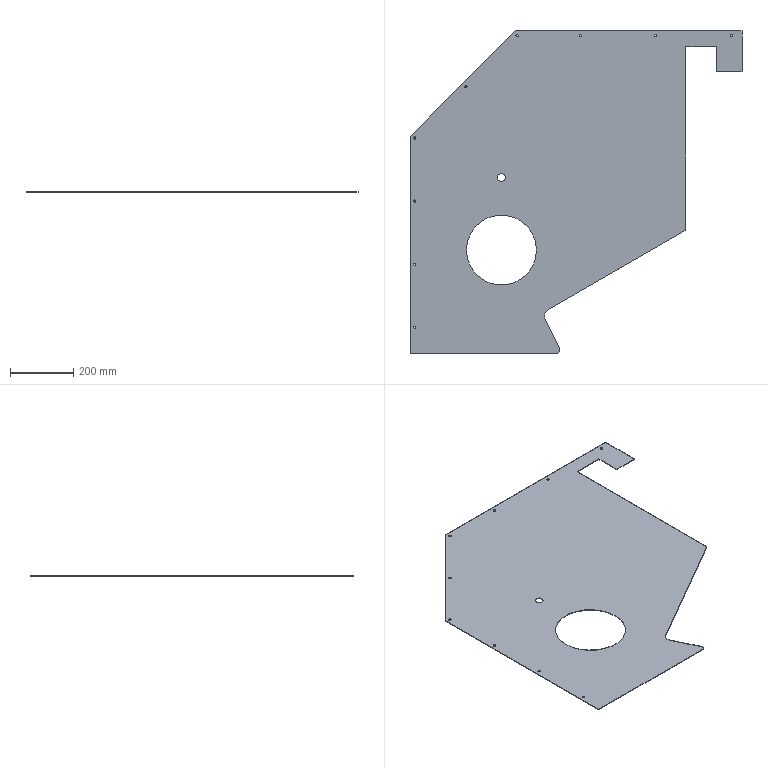Part | STEP file | Center Shaft Plate 2 | 1 solid | 38 faces | box 1053 x 1022 x 2 mm | volume 1400799 mm3 | cylinder 25 | plane 13 | commonest cylinder face diameters 7 x18 20 x2 25 x2 222 x2 40 x1
STEP:
#1=CARTESIAN_POINT('',(-529.64,-129.457,-2.));
#2=VERTEX_POINT('',#1);
#3=CARTESIAN_POINT('',(-519.64,-119.457,-2.));
#4=VERTEX_POINT('',#3);
#5=CARTESIAN_POINT('',(-529.64,-119.457,-2.));
#6=DIRECTION('',(0.,0.,1.));
#7=DIRECTION('',(1.,0.,0.));
#8=AXIS2_PLACEMENT_3D('',#5,#6,#7);
#9=CIRCLE('',#8,10.);
#10=EDGE_CURVE('',#2,#4,#9,.T.);
#11=ORIENTED_EDGE('',*,*,#10,.T.);
#12=CARTESIAN_POINT('',(-519.64,-119.457,0.));
#13=VERTEX_POINT('',#12);
#14=CARTESIAN_POINT('',(-519.64,-119.457,-2.));
#15=DIRECTION('',(0.,0.,1.));
#16=VECTOR('',#15,1000.);
#17=LINE('',#14,#16);
#18=EDGE_CURVE('',#4,#13,#17,.T.);
#19=ORIENTED_EDGE('',*,*,#18,.T.);
#20=CARTESIAN_POINT('',(-529.64,-129.457,0.));
#21=VERTEX_POINT('',#20);
#22=CARTESIAN_POINT('',(-529.64,-119.457,0.));
#23=DIRECTION('',(0.,0.,1.));
#24=DIRECTION('',(1.,0.,0.));
#25=AXIS2_PLACEMENT_3D('',#22,#23,#24);
#26=CIRCLE('',#25,10.);
#27=EDGE_CURVE('',#21,#13,#26,.T.);
#28=ORIENTED_EDGE('',*,*,#27,.F.);
#29=CARTESIAN_POINT('',(-529.64,-129.457,-2.));
#30=DIRECTION('',(0.,0.,-1.));
#31=VECTOR('',#30,1000.);
#32=LINE('',#29,#31);
#33=EDGE_CURVE('',#21,#2,#32,.T.);
#34=ORIENTED_EDGE('',*,*,#33,.T.);
#35=EDGE_LOOP('',(#11,#19,#28,#34));
#36=FACE_OUTER_BOUND('',#35,.T.);
#37=CARTESIAN_POINT('',(-529.64,-119.457,-2.));
#38=DIRECTION('',(0.,0.,1.));
#39=DIRECTION('',(1.,0.,0.));
#40=AXIS2_PLACEMENT_3D('',#37,#38,#39);
#41=CYLINDRICAL_SURFACE('',#40,10.);
#42=ADVANCED_FACE('',(#36),#41,.T.);
#43=CARTESIAN_POINT('',(-815.802,197.43,-2.));
#44=VERTEX_POINT('',#43);
#45=CARTESIAN_POINT('',(-593.802,197.43,-2.));
#46=VERTEX_POINT('',#45);
#47=CARTESIAN_POINT('',(-704.802,197.43,-2.));
#48=DIRECTION('',(0.,0.,1.));
#49=DIRECTION('',(1.,0.,0.));
#50=AXIS2_PLACEMENT_3D('',#47,#48,#49);
#51=CIRCLE('',#50,111.);
#52=EDGE_CURVE('',#44,#46,#51,.T.);
#53=ORIENTED_EDGE('',*,*,#52,.F.);
#54=CARTESIAN_POINT('',(-815.802,197.43,0.));
#55=VERTEX_POINT('',#54);
#56=CARTESIAN_POINT('',(-815.802,197.43,-2.));
#57=DIRECTION('',(0.,0.,1.));
#58=VECTOR('',#57,1000.);
#59=LINE('',#56,#58);
#60=EDGE_CURVE('',#44,#55,#59,.T.);
#61=ORIENTED_EDGE('',*,*,#60,.T.);
#62=CARTESIAN_POINT('',(-593.802,197.43,0.));
#63=VERTEX_POINT('',#62);
#64=CARTESIAN_POINT('',(-704.802,197.43,0.));
#65=DIRECTION('',(0.,0.,-1.));
#66=DIRECTION('',(1.,0.,0.));
#67=AXIS2_PLACEMENT_3D('',#64,#65,#66);
#68=CIRCLE('',#67,111.);
#69=EDGE_CURVE('',#63,#55,#68,.T.);
#70=ORIENTED_EDGE('',*,*,#69,.F.);
#71=CARTESIAN_POINT('',(-593.802,197.43,-2.));
#72=DIRECTION('',(0.,0.,1.));
#73=VECTOR('',#72,1000.);
#74=LINE('',#71,#73);
#75=EDGE_CURVE('',#46,#63,#74,.T.);
#76=ORIENTED_EDGE('',*,*,#75,.F.);
#77=EDGE_LOOP('',(#53,#61,#70,#76));
#78=FACE_OUTER_BOUND('',#77,.T.);
#79=CARTESIAN_POINT('',(-704.802,197.43,-2.));
#80=DIRECTION('',(0.,0.,1.));
#81=DIRECTION('',(1.,0.,0.));
#82=AXIS2_PLACEMENT_3D('',#79,#80,#81);
#83=CYLINDRICAL_SURFACE('',#82,111.);
#84=ADVANCED_FACE('',(#78),#83,.F.);
#85=CARTESIAN_POINT('',(-717.302,427.43,-2.));
#86=VERTEX_POINT('',#85);
#87=CARTESIAN_POINT('',(-692.302,427.43,-2.));
#88=VERTEX_POINT('',#87);
#89=CARTESIAN_POINT('',(-704.802,427.43,-2.));
#90=DIRECTION('',(0.,0.,1.));
#91=DIRECTION('',(1.,0.,0.));
#92=AXIS2_PLACEMENT_3D('',#89,#90,#91);
#93=CIRCLE('',#92,12.5);
#94=EDGE_CURVE('',#86,#88,#93,.T.);
#95=ORIENTED_EDGE('',*,*,#94,.F.);
#96=CARTESIAN_POINT('',(-717.302,427.43,0.));
#97=VERTEX_POINT('',#96);
#98=CARTESIAN_POINT('',(-717.302,427.43,-2.));
#99=DIRECTION('',(0.,0.,1.));
#100=VECTOR('',#99,1000.);
#101=LINE('',#98,#100);
#102=EDGE_CURVE('',#86,#97,#101,.T.);
#103=ORIENTED_EDGE('',*,*,#102,.T.);
#104=CARTESIAN_POINT('',(-692.302,427.43,0.));
#105=VERTEX_POINT('',#104);
#106=CARTESIAN_POINT('',(-704.802,427.43,0.));
#107=DIRECTION('',(0.,0.,-1.));
#108=DIRECTION('',(1.,0.,0.));
#109=AXIS2_PLACEMENT_3D('',#106,#107,#108);
#110=CIRCLE('',#109,12.5);
#111=EDGE_CURVE('',#105,#97,#110,.T.);
#112=ORIENTED_EDGE('',*,*,#111,.F.);
#113=CARTESIAN_POINT('',(-692.302,427.43,-2.));
#114=DIRECTION('',(0.,0.,1.));
#115=VECTOR('',#114,1000.);
#116=LINE('',#113,#115);
#117=EDGE_CURVE('',#88,#105,#116,.T.);
#118=ORIENTED_EDGE('',*,*,#117,.F.);
#119=EDGE_LOOP('',(#95,#103,#112,#118));
#120=FACE_OUTER_BOUND('',#119,.T.);
#121=CARTESIAN_POINT('',(-704.802,427.43,-2.));
#122=DIRECTION('',(0.,0.,1.));
#123=DIRECTION('',(1.,0.,0.));
#124=AXIS2_PLACEMENT_3D('',#121,#122,#123);
#125=CYLINDRICAL_SURFACE('',#124,12.5);
#126=ADVANCED_FACE('',(#120),#125,.F.);
#127=CARTESIAN_POINT('',(-983.302,552.785,-2.));
#128=VERTEX_POINT('',#127);
#129=CARTESIAN_POINT('',(-976.302,552.785,-2.));
#130=VERTEX_POINT('',#129);
#131=CARTESIAN_POINT('',(-979.802,552.785,-2.));
#132=DIRECTION('',(0.,0.,1.));
#133=DIRECTION('',(1.,0.,0.));
#134=AXIS2_PLACEMENT_3D('',#131,#132,#133);
#135=CIRCLE('',#134,3.5);
#136=EDGE_CURVE('',#128,#130,#135,.T.);
#137=ORIENTED_EDGE('',*,*,#136,.F.);
#138=CARTESIAN_POINT('',(-983.302,552.785,0.));
#139=VERTEX_POINT('',#138);
#140=CARTESIAN_POINT('',(-983.302,552.785,-10.));
#141=DIRECTION('',(0.,0.,1.));
#142=VECTOR('',#141,1000.);
#143=LINE('',#140,#142);
#144=EDGE_CURVE('',#128,#139,#143,.T.);
#145=ORIENTED_EDGE('',*,*,#144,.T.);
#146=CARTESIAN_POINT('',(-976.302,552.785,0.));
#147=VERTEX_POINT('',#146);
#148=CARTESIAN_POINT('',(-979.802,552.785,0.));
#149=DIRECTION('',(0.,0.,-1.));
#150=DIRECTION('',(1.,0.,0.));
#151=AXIS2_PLACEMENT_3D('',#148,#149,#150);
#152=CIRCLE('',#151,3.5);
#153=EDGE_CURVE('',#147,#139,#152,.T.);
#154=ORIENTED_EDGE('',*,*,#153,.F.);
#155=CARTESIAN_POINT('',(-976.302,552.785,-10.));
#156=DIRECTION('',(0.,0.,1.));
#157=VECTOR('',#156,1000.);
#158=LINE('',#155,#157);
#159=EDGE_CURVE('',#130,#147,#158,.T.);
#160=ORIENTED_EDGE('',*,*,#159,.F.);
#161=EDGE_LOOP('',(#137,#145,#154,#160));
#162=FACE_OUTER_BOUND('',#161,.T.);
#163=CARTESIAN_POINT('',(-979.802,552.785,-10.));
#164=DIRECTION('',(0.,0.,1.));
#165=DIRECTION('',(1.,0.,0.));
#166=AXIS2_PLACEMENT_3D('',#163,#164,#165);
#167=CYLINDRICAL_SURFACE('',#166,3.5);
#168=ADVANCED_FACE('',(#162),#167,.F.);
#169=CARTESIAN_POINT('',(-983.302,-47.215,-2.));
#170=VERTEX_POINT('',#169);
#171=CARTESIAN_POINT('',(-976.302,-47.215,-2.));
#172=VERTEX_POINT('',#171);
#173=CARTESIAN_POINT('',(-979.802,-47.215,-2.));
#174=DIRECTION('',(0.,0.,1.));
#175=DIRECTION('',(1.,0.,0.));
#176=AXIS2_PLACEMENT_3D('',#173,#174,#175);
#177=CIRCLE('',#176,3.5);
#178=EDGE_CURVE('',#170,#172,#177,.T.);
#179=ORIENTED_EDGE('',*,*,#178,.F.);
#180=CARTESIAN_POINT('',(-983.302,-47.215,0.));
#181=VERTEX_POINT('',#180);
#182=CARTESIAN_POINT('',(-983.302,-47.215,-10.));
#183=DIRECTION('',(0.,0.,1.));
#184=VECTOR('',#183,1000.);
#185=LINE('',#182,#184);
#186=EDGE_CURVE('',#170,#181,#185,.T.);
#187=ORIENTED_EDGE('',*,*,#186,.T.);
#188=CARTESIAN_POINT('',(-976.302,-47.215,0.));
#189=VERTEX_POINT('',#188);
#190=CARTESIAN_POINT('',(-979.802,-47.215,0.));
#191=DIRECTION('',(0.,0.,-1.));
#192=DIRECTION('',(1.,0.,0.));
#193=AXIS2_PLACEMENT_3D('',#190,#191,#192);
#194=CIRCLE('',#193,3.5);
#195=EDGE_CURVE('',#189,#181,#194,.T.);
#196=ORIENTED_EDGE('',*,*,#195,.F.);
#197=CARTESIAN_POINT('',(-976.302,-47.215,-10.));
#198=DIRECTION('',(0.,0.,1.));
#199=VECTOR('',#198,1000.);
#200=LINE('',#197,#199);
#201=EDGE_CURVE('',#172,#189,#200,.T.);
#202=ORIENTED_EDGE('',*,*,#201,.F.);
#203=EDGE_LOOP('',(#179,#187,#196,#202));
#204=FACE_OUTER_BOUND('',#203,.T.);
#205=CARTESIAN_POINT('',(-979.802,-47.215,-10.));
#206=DIRECTION('',(0.,0.,1.));
#207=DIRECTION('',(1.,0.,0.));
#208=AXIS2_PLACEMENT_3D('',#205,#206,#207);
#209=CYLINDRICAL_SURFACE('',#208,3.5);
#210=ADVANCED_FACE('',(#204),#209,.F.);
#211=CARTESIAN_POINT('',(-983.302,152.785,-2.));
#212=VERTEX_POINT('',#211);
#213=CARTESIAN_POINT('',(-976.302,152.785,-2.));
#214=VERTEX_POINT('',#213);
#215=CARTESIAN_POINT('',(-979.802,152.785,-2.));
#216=DIRECTION('',(0.,0.,1.));
#217=DIRECTION('',(1.,0.,0.));
#218=AXIS2_PLACEMENT_3D('',#215,#216,#217);
#219=CIRCLE('',#218,3.5);
#220=EDGE_CURVE('',#212,#214,#219,.T.);
#221=ORIENTED_EDGE('',*,*,#220,.F.);
#222=CARTESIAN_POINT('',(-983.302,152.785,0.));
#223=VERTEX_POINT('',#222);
#224=CARTESIAN_POINT('',(-983.302,152.785,-10.));
#225=DIRECTION('',(0.,0.,1.));
#226=VECTOR('',#225,1000.);
#227=LINE('',#224,#226);
#228=EDGE_CURVE('',#212,#223,#227,.T.);
#229=ORIENTED_EDGE('',*,*,#228,.T.);
#230=CARTESIAN_POINT('',(-976.302,152.785,0.));
#231=VERTEX_POINT('',#230);
#232=CARTESIAN_POINT('',(-979.802,152.785,0.));
#233=DIRECTION('',(0.,0.,-1.));
#234=DIRECTION('',(1.,0.,0.));
#235=AXIS2_PLACEMENT_3D('',#232,#233,#234);
#236=CIRCLE('',#235,3.5);
#237=EDGE_CURVE('',#231,#223,#236,.T.);
#238=ORIENTED_EDGE('',*,*,#237,.F.);
#239=CARTESIAN_POINT('',(-976.302,152.785,-10.));
#240=DIRECTION('',(0.,0.,1.));
#241=VECTOR('',#240,1000.);
#242=LINE('',#239,#241);
#243=EDGE_CURVE('',#214,#231,#242,.T.);
#244=ORIENTED_EDGE('',*,*,#243,.F.);
#245=EDGE_LOOP('',(#221,#229,#238,#244));
#246=FACE_OUTER_BOUND('',#245,.T.);
#247=CARTESIAN_POINT('',(-979.802,152.785,-10.));
#248=DIRECTION('',(0.,0.,1.));
#249=DIRECTION('',(1.,0.,0.));
#250=AXIS2_PLACEMENT_3D('',#247,#248,#249);
#251=CYLINDRICAL_SURFACE('',#250,3.5);
#252=ADVANCED_FACE('',(#246),#251,.F.);
#253=CARTESIAN_POINT('',(-983.302,352.785,-2.));
#254=VERTEX_POINT('',#253);
#255=CARTESIAN_POINT('',(-976.302,352.785,-2.));
#256=VERTEX_POINT('',#255);
#257=CARTESIAN_POINT('',(-979.802,352.785,-2.));
#258=DIRECTION('',(0.,0.,1.));
#259=DIRECTION('',(1.,0.,0.));
#260=AXIS2_PLACEMENT_3D('',#257,#258,#259);
#261=CIRCLE('',#260,3.5);
#262=EDGE_CURVE('',#254,#256,#261,.T.);
#263=ORIENTED_EDGE('',*,*,#262,.F.);
#264=CARTESIAN_POINT('',(-983.302,352.785,0.));
#265=VERTEX_POINT('',#264);
#266=CARTESIAN_POINT('',(-983.302,352.785,-10.));
#267=DIRECTION('',(0.,0.,1.));
#268=VECTOR('',#267,1000.);
#269=LINE('',#266,#268);
#270=EDGE_CURVE('',#254,#265,#269,.T.);
#271=ORIENTED_EDGE('',*,*,#270,.T.);
#272=CARTESIAN_POINT('',(-976.302,352.785,0.));
#273=VERTEX_POINT('',#272);
#274=CARTESIAN_POINT('',(-979.802,352.785,0.));
#275=DIRECTION('',(0.,0.,-1.));
#276=DIRECTION('',(1.,0.,0.));
#277=AXIS2_PLACEMENT_3D('',#274,#275,#276);
#278=CIRCLE('',#277,3.5);
#279=EDGE_CURVE('',#273,#265,#278,.T.);
#280=ORIENTED_EDGE('',*,*,#279,.F.);
#281=CARTESIAN_POINT('',(-976.302,352.785,-10.));
#282=DIRECTION('',(0.,0.,1.));
#283=VECTOR('',#282,1000.);
#284=LINE('',#281,#283);
#285=EDGE_CURVE('',#256,#273,#284,.T.);
#286=ORIENTED_EDGE('',*,*,#285,.F.);
#287=EDGE_LOOP('',(#263,#271,#280,#286));
#288=FACE_OUTER_BOUND('',#287,.T.);
#289=CARTESIAN_POINT('',(-979.802,352.785,-10.));
#290=DIRECTION('',(0.,0.,1.));
#291=DIRECTION('',(1.,0.,0.));
#292=AXIS2_PLACEMENT_3D('',#289,#290,#291);
#293=CYLINDRICAL_SURFACE('',#292,3.5);
#294=ADVANCED_FACE('',(#288),#293,.F.);
#295=CARTESIAN_POINT('',(-658.658,877.43,-2.));
#296=VERTEX_POINT('',#295);
#297=CARTESIAN_POINT('',(-651.658,877.43,-2.));
#298=VERTEX_POINT('',#297);
#299=CARTESIAN_POINT('',(-655.158,877.43,-2.));
#300=DIRECTION('',(0.,0.,1.));
#301=DIRECTION('',(1.,0.,0.));
#302=AXIS2_PLACEMENT_3D('',#299,#300,#301);
#303=CIRCLE('',#302,3.5);
#304=EDGE_CURVE('',#296,#298,#303,.T.);
#305=ORIENTED_EDGE('',*,*,#304,.F.);
#306=CARTESIAN_POINT('',(-658.658,877.43,0.));
#307=VERTEX_POINT('',#306);
#308=CARTESIAN_POINT('',(-658.658,877.43,-10.));
#309=DIRECTION('',(0.,0.,1.));
#310=VECTOR('',#309,1000.);
#311=LINE('',#308,#310);
#312=EDGE_CURVE('',#296,#307,#311,.T.);
#313=ORIENTED_EDGE('',*,*,#312,.T.);
#314=CARTESIAN_POINT('',(-651.658,877.43,0.));
#315=VERTEX_POINT('',#314);
#316=CARTESIAN_POINT('',(-655.158,877.43,0.));
#317=DIRECTION('',(0.,0.,-1.));
#318=DIRECTION('',(1.,0.,0.));
#319=AXIS2_PLACEMENT_3D('',#316,#317,#318);
#320=CIRCLE('',#319,3.5);
#321=EDGE_CURVE('',#315,#307,#320,.T.);
#322=ORIENTED_EDGE('',*,*,#321,.F.);
#323=CARTESIAN_POINT('',(-651.658,877.43,-10.));
#324=DIRECTION('',(0.,0.,1.));
#325=VECTOR('',#324,1000.);
#326=LINE('',#323,#325);
#327=EDGE_CURVE('',#298,#315,#326,.T.);
#328=ORIENTED_EDGE('',*,*,#327,.F.);
#329=EDGE_LOOP('',(#305,#313,#322,#328));
#330=FACE_OUTER_BOUND('',#329,.T.);
#331=CARTESIAN_POINT('',(-655.158,877.43,-10.));
#332=DIRECTION('',(0.,0.,1.));
#333=DIRECTION('',(1.,0.,0.));
#334=AXIS2_PLACEMENT_3D('',#331,#332,#333);
#335=CYLINDRICAL_SURFACE('',#334,3.5);
#336=ADVANCED_FACE('',(#330),#335,.F.);
#337=CARTESIAN_POINT('',(-820.98,715.107,-2.));
#338=VERTEX_POINT('',#337);
#339=CARTESIAN_POINT('',(-813.98,715.107,-2.));
#340=VERTEX_POINT('',#339);
#341=CARTESIAN_POINT('',(-817.48,715.107,-2.));
#342=DIRECTION('',(0.,0.,1.));
#343=DIRECTION('',(1.,0.,0.));
#344=AXIS2_PLACEMENT_3D('',#341,#342,#343);
#345=CIRCLE('',#344,3.5);
#346=EDGE_CURVE('',#338,#340,#345,.T.);
#347=ORIENTED_EDGE('',*,*,#346,.F.);
#348=CARTESIAN_POINT('',(-820.98,715.107,0.));
#349=VERTEX_POINT('',#348);
#350=CARTESIAN_POINT('',(-820.98,715.107,-10.));
#351=DIRECTION('',(0.,0.,1.));
#352=VECTOR('',#351,1000.);
#353=LINE('',#350,#352);
#354=EDGE_CURVE('',#338,#349,#353,.T.);
#355=ORIENTED_EDGE('',*,*,#354,.T.);
#356=CARTESIAN_POINT('',(-813.98,715.107,0.));
#357=VERTEX_POINT('',#356);
#358=CARTESIAN_POINT('',(-817.48,715.107,0.));
#359=DIRECTION('',(0.,0.,-1.));
#360=DIRECTION('',(1.,0.,0.));
#361=AXIS2_PLACEMENT_3D('',#358,#359,#360);
#362=CIRCLE('',#361,3.5);
#363=EDGE_CURVE('',#357,#349,#362,.T.);
#364=ORIENTED_EDGE('',*,*,#363,.F.);
#365=CARTESIAN_POINT('',(-813.98,715.107,-10.));
#366=DIRECTION('',(0.,0.,1.));
#367=VECTOR('',#366,1000.);
#368=LINE('',#365,#367);
#369=EDGE_CURVE('',#340,#357,#368,.T.);
#370=ORIENTED_EDGE('',*,*,#369,.F.);
#371=EDGE_LOOP('',(#347,#355,#364,#370));
#372=FACE_OUTER_BOUND('',#371,.T.);
#373=CARTESIAN_POINT('',(-817.48,715.107,-10.));
#374=DIRECTION('',(0.,0.,1.));
#375=DIRECTION('',(1.,0.,0.));
#376=AXIS2_PLACEMENT_3D('',#373,#374,#375);
#377=CYLINDRICAL_SURFACE('',#376,3.5);
#378=ADVANCED_FACE('',(#372),#377,.F.);
#379=CARTESIAN_POINT('',(-458.658,877.43,-2.));
#380=VERTEX_POINT('',#379);
#381=CARTESIAN_POINT('',(-451.658,877.43,-2.));
#382=VERTEX_POINT('',#381);
#383=CARTESIAN_POINT('',(-455.158,877.43,-2.));
#384=DIRECTION('',(0.,0.,1.));
#385=DIRECTION('',(1.,0.,0.));
#386=AXIS2_PLACEMENT_3D('',#383,#384,#385);
#387=CIRCLE('',#386,3.5);
#388=EDGE_CURVE('',#380,#382,#387,.T.);
#389=ORIENTED_EDGE('',*,*,#388,.F.);
#390=CARTESIAN_POINT('',(-458.658,877.43,0.));
#391=VERTEX_POINT('',#390);
#392=CARTESIAN_POINT('',(-458.658,877.43,-10.));
#393=DIRECTION('',(0.,0.,1.));
#394=VECTOR('',#393,1000.);
#395=LINE('',#392,#394);
#396=EDGE_CURVE('',#380,#391,#395,.T.);
#397=ORIENTED_EDGE('',*,*,#396,.T.);
#398=CARTESIAN_POINT('',(-451.658,877.43,0.));
#399=VERTEX_POINT('',#398);
#400=CARTESIAN_POINT('',(-455.158,877.43,0.));
#401=DIRECTION('',(0.,0.,-1.));
#402=DIRECTION('',(1.,0.,0.));
#403=AXIS2_PLACEMENT_3D('',#400,#401,#402);
#404=CIRCLE('',#403,3.5);
#405=EDGE_CURVE('',#399,#391,#404,.T.);
#406=ORIENTED_EDGE('',*,*,#405,.F.);
#407=CARTESIAN_POINT('',(-451.658,877.43,-10.));
#408=DIRECTION('',(0.,0.,1.));
#409=VECTOR('',#408,1000.);
#410=LINE('',#407,#409);
#411=EDGE_CURVE('',#382,#399,#410,.T.);
#412=ORIENTED_EDGE('',*,*,#411,.F.);
#413=EDGE_LOOP('',(#389,#397,#406,#412));
#414=FACE_OUTER_BOUND('',#413,.T.);
#415=CARTESIAN_POINT('',(-455.158,877.43,-10.));
#416=DIRECTION('',(0.,0.,1.));
#417=DIRECTION('',(1.,0.,0.));
#418=AXIS2_PLACEMENT_3D('',#415,#416,#417);
#419=CYLINDRICAL_SURFACE('',#418,3.5);
#420=ADVANCED_FACE('',(#414),#419,.F.);
#421=CARTESIAN_POINT('',(-218.658,877.43,-2.));
#422=VERTEX_POINT('',#421);
#423=CARTESIAN_POINT('',(-211.658,877.43,-2.));
#424=VERTEX_POINT('',#423);
#425=CARTESIAN_POINT('',(-215.158,877.43,-2.));
#426=DIRECTION('',(0.,0.,1.));
#427=DIRECTION('',(1.,0.,0.));
#428=AXIS2_PLACEMENT_3D('',#425,#426,#427);
#429=CIRCLE('',#428,3.5);
#430=EDGE_CURVE('',#422,#424,#429,.T.);
#431=ORIENTED_EDGE('',*,*,#430,.F.);
#432=CARTESIAN_POINT('',(-218.658,877.43,0.));
#433=VERTEX_POINT('',#432);
#434=CARTESIAN_POINT('',(-218.658,877.43,-10.));
#435=DIRECTION('',(0.,0.,1.));
#436=VECTOR('',#435,1000.);
#437=LINE('',#434,#436);
#438=EDGE_CURVE('',#422,#433,#437,.T.);
#439=ORIENTED_EDGE('',*,*,#438,.T.);
#440=CARTESIAN_POINT('',(-211.658,877.43,0.));
#441=VERTEX_POINT('',#440);
#442=CARTESIAN_POINT('',(-215.158,877.43,0.));
#443=DIRECTION('',(0.,0.,-1.));
#444=DIRECTION('',(1.,0.,0.));
#445=AXIS2_PLACEMENT_3D('',#442,#443,#444);
#446=CIRCLE('',#445,3.5);
#447=EDGE_CURVE('',#441,#433,#446,.T.);
#448=ORIENTED_EDGE('',*,*,#447,.F.);
#449=CARTESIAN_POINT('',(-211.658,877.43,-10.));
#450=DIRECTION('',(0.,0.,1.));
#451=VECTOR('',#450,1000.);
#452=LINE('',#449,#451);
#453=EDGE_CURVE('',#424,#441,#452,.T.);
#454=ORIENTED_EDGE('',*,*,#453,.F.);
#455=EDGE_LOOP('',(#431,#439,#448,#454));
#456=FACE_OUTER_BOUND('',#455,.T.);
#457=CARTESIAN_POINT('',(-215.158,877.43,-10.));
#458=DIRECTION('',(0.,0.,1.));
#459=DIRECTION('',(1.,0.,0.));
#460=AXIS2_PLACEMENT_3D('',#457,#458,#459);
#461=CYLINDRICAL_SURFACE('',#460,3.5);
#462=ADVANCED_FACE('',(#456),#461,.F.);
#463=CARTESIAN_POINT('',(21.342,877.43,-2.));
#464=VERTEX_POINT('',#463);
#465=CARTESIAN_POINT('',(28.342,877.43,-2.));
#466=VERTEX_POINT('',#465);
#467=CARTESIAN_POINT('',(24.842,877.43,-2.));
#468=DIRECTION('',(0.,0.,1.));
#469=DIRECTION('',(1.,0.,0.));
#470=AXIS2_PLACEMENT_3D('',#467,#468,#469);
#471=CIRCLE('',#470,3.5);
#472=EDGE_CURVE('',#464,#466,#471,.T.);
#473=ORIENTED_EDGE('',*,*,#472,.F.);
#474=CARTESIAN_POINT('',(21.342,877.43,0.));
#475=VERTEX_POINT('',#474);
#476=CARTESIAN_POINT('',(21.342,877.43,-10.));
#477=DIRECTION('',(0.,0.,1.));
#478=VECTOR('',#477,1000.);
#479=LINE('',#476,#478);
#480=EDGE_CURVE('',#464,#475,#479,.T.);
#481=ORIENTED_EDGE('',*,*,#480,.T.);
#482=CARTESIAN_POINT('',(28.342,877.43,0.));
#483=VERTEX_POINT('',#482);
#484=CARTESIAN_POINT('',(24.842,877.43,0.));
#485=DIRECTION('',(0.,0.,-1.));
#486=DIRECTION('',(1.,0.,0.));
#487=AXIS2_PLACEMENT_3D('',#484,#485,#486);
#488=CIRCLE('',#487,3.5);
#489=EDGE_CURVE('',#483,#475,#488,.T.);
#490=ORIENTED_EDGE('',*,*,#489,.F.);
#491=CARTESIAN_POINT('',(28.342,877.43,-10.));
#492=DIRECTION('',(0.,0.,1.));
#493=VECTOR('',#492,1000.);
#494=LINE('',#491,#493);
#495=EDGE_CURVE('',#466,#483,#494,.T.);
#496=ORIENTED_EDGE('',*,*,#495,.F.);
#497=EDGE_LOOP('',(#473,#481,#490,#496));
#498=FACE_OUTER_BOUND('',#497,.T.);
#499=CARTESIAN_POINT('',(24.842,877.43,-10.));
#500=DIRECTION('',(0.,0.,1.));
#501=DIRECTION('',(1.,0.,0.));
#502=AXIS2_PLACEMENT_3D('',#499,#500,#501);
#503=CYLINDRICAL_SURFACE('',#502,3.5);
#504=ADVANCED_FACE('',(#498),#503,.F.);
#505=CARTESIAN_POINT('',(-661.371,892.43,0.));
#506=VERTEX_POINT('',#505);
#507=CARTESIAN_POINT('',(-994.802,558.998,0.));
#508=VERTEX_POINT('',#507);
#509=CARTESIAN_POINT('',(-661.371,892.43,0.));
#510=DIRECTION('',(-0.7071,-0.7071,0.));
#511=VECTOR('',#510,1000.);
#512=LINE('',#509,#511);
#513=EDGE_CURVE('',#506,#508,#512,.T.);
#514=ORIENTED_EDGE('',*,*,#513,.T.);
#515=CARTESIAN_POINT('',(-994.802,-129.457,0.));
#516=VERTEX_POINT('',#515);
#517=CARTESIAN_POINT('',(-994.802,-10.278,0.));
#518=DIRECTION('',(0.,-1.,0.));
#519=VECTOR('',#518,1000.);
#520=LINE('',#517,#519);
#521=EDGE_CURVE('',#508,#516,#520,.T.);
#522=ORIENTED_EDGE('',*,*,#521,.T.);
#523=CARTESIAN_POINT('',(-548.641,-129.457,0.));
#524=DIRECTION('',(1.,0.,0.));
#525=VECTOR('',#524,1000.);
#526=LINE('',#523,#525);
#527=EDGE_CURVE('',#516,#21,#526,.T.);
#528=ORIENTED_EDGE('',*,*,#527,.T.);
#529=ORIENTED_EDGE('',*,*,#27,.T.);
#530=CARTESIAN_POINT('',(-520.62,-115.139,0.));
#531=VERTEX_POINT('',#530);
#532=CARTESIAN_POINT('',(-529.64,-119.457,0.));
#533=DIRECTION('',(0.,0.,1.));
#534=DIRECTION('',(1.,0.,0.));
#535=AXIS2_PLACEMENT_3D('',#532,#533,#534);
#536=CIRCLE('',#535,10.);
#537=EDGE_CURVE('',#13,#531,#536,.T.);
#538=ORIENTED_EDGE('',*,*,#537,.T.);
#539=CARTESIAN_POINT('',(-566.68,-18.913,0.));
#540=VERTEX_POINT('',#539);
#541=CARTESIAN_POINT('',(-520.62,-115.139,0.));
#542=DIRECTION('',(-0.4318,0.902,0.));
#543=VECTOR('',#542,1000.);
#544=LINE('',#541,#543);
#545=EDGE_CURVE('',#531,#540,#544,.T.);
#546=ORIENTED_EDGE('',*,*,#545,.T.);
#547=CARTESIAN_POINT('',(-558.641,7.042,0.));
#548=VERTEX_POINT('',#547);
#549=CARTESIAN_POINT('',(-548.641,-10.278,0.));
#550=DIRECTION('',(0.,0.,-1.));
#551=DIRECTION('',(1.,0.,0.));
#552=AXIS2_PLACEMENT_3D('',#549,#550,#551);
#553=CIRCLE('',#552,20.);
#554=EDGE_CURVE('',#540,#548,#553,.T.);
#555=ORIENTED_EDGE('',*,*,#554,.T.);
#556=CARTESIAN_POINT('',(-120.132,260.215,0.));
#557=VERTEX_POINT('',#556);
#558=CARTESIAN_POINT('',(-558.641,7.042,0.));
#559=DIRECTION('',(0.866,0.5,0.));
#560=VECTOR('',#559,1000.);
#561=LINE('',#558,#560);
#562=EDGE_CURVE('',#548,#557,#561,.T.);
#563=ORIENTED_EDGE('',*,*,#562,.T.);
#564=CARTESIAN_POINT('',(-120.132,842.43,0.));
#565=VERTEX_POINT('',#564);
#566=CARTESIAN_POINT('',(-120.132,-10.278,0.));
#567=DIRECTION('',(0.,1.,0.));
#568=VECTOR('',#567,1000.);
#569=LINE('',#566,#568);
#570=EDGE_CURVE('',#557,#565,#569,.T.);
#571=ORIENTED_EDGE('',*,*,#570,.T.);
#572=CARTESIAN_POINT('',(-21.932,842.43,0.));
#573=VERTEX_POINT('',#572);
#574=CARTESIAN_POINT('',(-548.641,842.43,0.));
#575=DIRECTION('',(1.,0.,0.));
#576=VECTOR('',#575,1000.);
#577=LINE('',#574,#576);
#578=EDGE_CURVE('',#565,#573,#577,.T.);
#579=ORIENTED_EDGE('',*,*,#578,.T.);
#580=CARTESIAN_POINT('',(-21.932,762.43,0.));
#581=VERTEX_POINT('',#580);
#582=CARTESIAN_POINT('',(-21.932,-10.278,0.));
#583=DIRECTION('',(0.,-1.,0.));
#584=VECTOR('',#583,1000.);
#585=LINE('',#582,#584);
#586=EDGE_CURVE('',#573,#581,#585,.T.);
#587=ORIENTED_EDGE('',*,*,#586,.T.);
#588=CARTESIAN_POINT('',(58.068,762.43,0.));
#589=VERTEX_POINT('',#588);
#590=CARTESIAN_POINT('',(-548.641,762.43,0.));
#591=DIRECTION('',(1.,0.,0.));
#592=VECTOR('',#591,1000.);
#593=LINE('',#590,#592);
#594=EDGE_CURVE('',#581,#589,#593,.T.);
#595=ORIENTED_EDGE('',*,*,#594,.T.);
#596=CARTESIAN_POINT('',(58.068,892.43,0.));
#597=VERTEX_POINT('',#596);
#598=CARTESIAN_POINT('',(58.068,-10.278,0.));
#599=DIRECTION('',(0.,1.,0.));
#600=VECTOR('',#599,1000.);
#601=LINE('',#598,#600);
#602=EDGE_CURVE('',#589,#597,#601,.T.);
#603=ORIENTED_EDGE('',*,*,#602,.T.);
#604=CARTESIAN_POINT('',(-548.641,892.43,0.));
#605=DIRECTION('',(-1.,0.,0.));
#606=VECTOR('',#605,1000.);
#607=LINE('',#604,#606);
#608=EDGE_CURVE('',#597,#506,#607,.T.);
#609=ORIENTED_EDGE('',*,*,#608,.T.);
#610=EDGE_LOOP('',(#514,#522,#528,#529,#538,#546,#555,#563,#571,#579,#587,#595,#603,#609));
#611=FACE_OUTER_BOUND('',#610,.T.);
#612=ORIENTED_EDGE('',*,*,#69,.T.);
#613=CARTESIAN_POINT('',(-704.802,197.43,0.));
#614=DIRECTION('',(0.,0.,-1.));
#615=DIRECTION('',(1.,0.,0.));
#616=AXIS2_PLACEMENT_3D('',#613,#614,#615);
#617=CIRCLE('',#616,111.);
#618=EDGE_CURVE('',#55,#63,#617,.T.);
#619=ORIENTED_EDGE('',*,*,#618,.T.);
#620=EDGE_LOOP('',(#612,#619));
#621=FACE_BOUND('',#620,.T.);
#622=ORIENTED_EDGE('',*,*,#111,.T.);
#623=CARTESIAN_POINT('',(-704.802,427.43,0.));
#624=DIRECTION('',(0.,0.,-1.));
#625=DIRECTION('',(1.,0.,0.));
#626=AXIS2_PLACEMENT_3D('',#623,#624,#625);
#627=CIRCLE('',#626,12.5);
#628=EDGE_CURVE('',#97,#105,#627,.T.);
#629=ORIENTED_EDGE('',*,*,#628,.T.);
#630=EDGE_LOOP('',(#622,#629));
#631=FACE_BOUND('',#630,.T.);
#632=ORIENTED_EDGE('',*,*,#153,.T.);
#633=CARTESIAN_POINT('',(-979.802,552.785,0.));
#634=DIRECTION('',(0.,0.,-1.));
#635=DIRECTION('',(1.,0.,0.));
#636=AXIS2_PLACEMENT_3D('',#633,#634,#635);
#637=CIRCLE('',#636,3.5);
#638=EDGE_CURVE('',#139,#147,#637,.T.);
#639=ORIENTED_EDGE('',*,*,#638,.T.);
#640=EDGE_LOOP('',(#632,#639));
#641=FACE_BOUND('',#640,.T.);
#642=ORIENTED_EDGE('',*,*,#195,.T.);
#643=CARTESIAN_POINT('',(-979.802,-47.215,0.));
#644=DIRECTION('',(0.,0.,-1.));
#645=DIRECTION('',(1.,0.,0.));
#646=AXIS2_PLACEMENT_3D('',#643,#644,#645);
#647=CIRCLE('',#646,3.5);
#648=EDGE_CURVE('',#181,#189,#647,.T.);
#649=ORIENTED_EDGE('',*,*,#648,.T.);
#650=EDGE_LOOP('',(#642,#649));
#651=FACE_BOUND('',#650,.T.);
#652=ORIENTED_EDGE('',*,*,#237,.T.);
#653=CARTESIAN_POINT('',(-979.802,152.785,0.));
#654=DIRECTION('',(0.,0.,-1.));
#655=DIRECTION('',(1.,0.,0.));
#656=AXIS2_PLACEMENT_3D('',#653,#654,#655);
#657=CIRCLE('',#656,3.5);
#658=EDGE_CURVE('',#223,#231,#657,.T.);
#659=ORIENTED_EDGE('',*,*,#658,.T.);
#660=EDGE_LOOP('',(#652,#659));
#661=FACE_BOUND('',#660,.T.);
#662=ORIENTED_EDGE('',*,*,#279,.T.);
#663=CARTESIAN_POINT('',(-979.802,352.785,0.));
#664=DIRECTION('',(0.,0.,-1.));
#665=DIRECTION('',(1.,0.,0.));
#666=AXIS2_PLACEMENT_3D('',#663,#664,#665);
#667=CIRCLE('',#666,3.5);
#668=EDGE_CURVE('',#265,#273,#667,.T.);
#669=ORIENTED_EDGE('',*,*,#668,.T.);
#670=EDGE_LOOP('',(#662,#669));
#671=FACE_BOUND('',#670,.T.);
#672=ORIENTED_EDGE('',*,*,#321,.T.);
#673=CARTESIAN_POINT('',(-655.158,877.43,0.));
#674=DIRECTION('',(0.,0.,-1.));
#675=DIRECTION('',(1.,0.,0.));
#676=AXIS2_PLACEMENT_3D('',#673,#674,#675);
#677=CIRCLE('',#676,3.5);
#678=EDGE_CURVE('',#307,#315,#677,.T.);
#679=ORIENTED_EDGE('',*,*,#678,.T.);
#680=EDGE_LOOP('',(#672,#679));
#681=FACE_BOUND('',#680,.T.);
#682=ORIENTED_EDGE('',*,*,#363,.T.);
#683=CARTESIAN_POINT('',(-817.48,715.107,0.));
#684=DIRECTION('',(0.,0.,-1.));
#685=DIRECTION('',(1.,0.,0.));
#686=AXIS2_PLACEMENT_3D('',#683,#684,#685);
#687=CIRCLE('',#686,3.5);
#688=EDGE_CURVE('',#349,#357,#687,.T.);
#689=ORIENTED_EDGE('',*,*,#688,.T.);
#690=EDGE_LOOP('',(#682,#689));
#691=FACE_BOUND('',#690,.T.);
#692=ORIENTED_EDGE('',*,*,#405,.T.);
#693=CARTESIAN_POINT('',(-455.158,877.43,0.));
#694=DIRECTION('',(0.,0.,-1.));
#695=DIRECTION('',(1.,0.,0.));
#696=AXIS2_PLACEMENT_3D('',#693,#694,#695);
#697=CIRCLE('',#696,3.5);
#698=EDGE_CURVE('',#391,#399,#697,.T.);
#699=ORIENTED_EDGE('',*,*,#698,.T.);
#700=EDGE_LOOP('',(#692,#699));
#701=FACE_BOUND('',#700,.T.);
#702=ORIENTED_EDGE('',*,*,#447,.T.);
#703=CARTESIAN_POINT('',(-215.158,877.43,0.));
#704=DIRECTION('',(0.,0.,-1.));
#705=DIRECTION('',(1.,0.,0.));
#706=AXIS2_PLACEMENT_3D('',#703,#704,#705);
#707=CIRCLE('',#706,3.5);
#708=EDGE_CURVE('',#433,#441,#707,.T.);
#709=ORIENTED_EDGE('',*,*,#708,.T.);
#710=EDGE_LOOP('',(#702,#709));
#711=FACE_BOUND('',#710,.T.);
#712=ORIENTED_EDGE('',*,*,#489,.T.);
#713=CARTESIAN_POINT('',(24.842,877.43,0.));
#714=DIRECTION('',(0.,0.,-1.));
#715=DIRECTION('',(1.,0.,0.));
#716=AXIS2_PLACEMENT_3D('',#713,#714,#715);
#717=CIRCLE('',#716,3.5);
#718=EDGE_CURVE('',#475,#483,#717,.T.);
#719=ORIENTED_EDGE('',*,*,#718,.T.);
#720=EDGE_LOOP('',(#712,#719));
#721=FACE_BOUND('',#720,.T.);
#722=CARTESIAN_POINT('',(-548.641,-10.278,0.));
#723=DIRECTION('',(0.,0.,1.));
#724=DIRECTION('',(1.,0.,0.));
#725=AXIS2_PLACEMENT_3D('',#722,#723,#724);
#726=PLANE('',#725);
#727=ADVANCED_FACE('',(#611,#621,#631,#641,#651,#661,#671,#681,#691,#701,#711,#721),#726,.T.);
#728=CARTESIAN_POINT('',(-994.802,558.998,-2.));
#729=VERTEX_POINT('',#728);
#730=CARTESIAN_POINT('',(-994.802,-129.457,-2.));
#731=VERTEX_POINT('',#730);
#732=CARTESIAN_POINT('',(-994.802,558.998,-2.));
#733=DIRECTION('',(0.,-1.,0.));
#734=VECTOR('',#733,1000.);
#735=LINE('',#732,#734);
#736=EDGE_CURVE('',#729,#731,#735,.T.);
#737=ORIENTED_EDGE('',*,*,#736,.T.);
#738=CARTESIAN_POINT('',(-994.802,-129.457,-2.));
#739=DIRECTION('',(0.,0.,1.));
#740=VECTOR('',#739,1000.);
#741=LINE('',#738,#740);
#742=EDGE_CURVE('',#731,#516,#741,.T.);
#743=ORIENTED_EDGE('',*,*,#742,.T.);
#744=ORIENTED_EDGE('',*,*,#521,.F.);
#745=CARTESIAN_POINT('',(-994.802,558.998,-2.));
#746=DIRECTION('',(0.,0.,-1.));
#747=VECTOR('',#746,1000.);
#748=LINE('',#745,#747);
#749=EDGE_CURVE('',#508,#729,#748,.T.);
#750=ORIENTED_EDGE('',*,*,#749,.T.);
#751=EDGE_LOOP('',(#737,#743,#744,#750));
#752=FACE_OUTER_BOUND('',#751,.T.);
#753=CARTESIAN_POINT('',(-994.802,558.998,-2.));
#754=DIRECTION('',(-1.,0.,0.));
#755=DIRECTION('',(0.,-1.,0.));
#756=AXIS2_PLACEMENT_3D('',#753,#754,#755);
#757=PLANE('',#756);
#758=ADVANCED_FACE('',(#752),#757,.T.);
#759=CARTESIAN_POINT('',(-661.371,892.43,-2.));
#760=VERTEX_POINT('',#759);
#761=CARTESIAN_POINT('',(-661.371,892.43,-2.));
#762=DIRECTION('',(-0.7071,-0.7071,0.));
#763=VECTOR('',#762,1000.);
#764=LINE('',#761,#763);
#765=EDGE_CURVE('',#760,#729,#764,.T.);
#766=ORIENTED_EDGE('',*,*,#765,.T.);
#767=ORIENTED_EDGE('',*,*,#749,.F.);
#768=ORIENTED_EDGE('',*,*,#513,.F.);
#769=CARTESIAN_POINT('',(-661.371,892.43,-2.));
#770=DIRECTION('',(0.,0.,-1.));
#771=VECTOR('',#770,1000.);
#772=LINE('',#769,#771);
#773=EDGE_CURVE('',#506,#760,#772,.T.);
#774=ORIENTED_EDGE('',*,*,#773,.T.);
#775=EDGE_LOOP('',(#766,#767,#768,#774));
#776=FACE_OUTER_BOUND('',#775,.T.);
#777=CARTESIAN_POINT('',(-661.371,892.43,-2.));
#778=DIRECTION('',(-0.7071,0.7071,0.));
#779=DIRECTION('',(-0.7071,-0.7071,0.));
#780=AXIS2_PLACEMENT_3D('',#777,#778,#779);
#781=PLANE('',#780);
#782=ADVANCED_FACE('',(#776),#781,.T.);
#783=CARTESIAN_POINT('',(58.068,892.43,-2.));
#784=VERTEX_POINT('',#783);
#785=CARTESIAN_POINT('',(58.068,892.43,-2.));
#786=DIRECTION('',(-1.,0.,0.));
#787=VECTOR('',#786,1000.);
#788=LINE('',#785,#787);
#789=EDGE_CURVE('',#784,#760,#788,.T.);
#790=ORIENTED_EDGE('',*,*,#789,.T.);
#791=ORIENTED_EDGE('',*,*,#773,.F.);
#792=ORIENTED_EDGE('',*,*,#608,.F.);
#793=CARTESIAN_POINT('',(58.068,892.43,-2.));
#794=DIRECTION('',(0.,0.,-1.));
#795=VECTOR('',#794,1000.);
#796=LINE('',#793,#795);
#797=EDGE_CURVE('',#597,#784,#796,.T.);
#798=ORIENTED_EDGE('',*,*,#797,.T.);
#799=EDGE_LOOP('',(#790,#791,#792,#798));
#800=FACE_OUTER_BOUND('',#799,.T.);
#801=CARTESIAN_POINT('',(58.068,892.43,-2.));
#802=DIRECTION('',(0.,1.,0.));
#803=DIRECTION('',(-1.,0.,0.));
#804=AXIS2_PLACEMENT_3D('',#801,#802,#803);
#805=PLANE('',#804);
#806=ADVANCED_FACE('',(#800),#805,.T.);
#807=CARTESIAN_POINT('',(58.068,762.43,-2.));
#808=VERTEX_POINT('',#807);
#809=CARTESIAN_POINT('',(58.068,762.43,-2.));
#810=DIRECTION('',(0.,1.,0.));
#811=VECTOR('',#810,1000.);
#812=LINE('',#809,#811);
#813=EDGE_CURVE('',#808,#784,#812,.T.);
#814=ORIENTED_EDGE('',*,*,#813,.T.);
#815=ORIENTED_EDGE('',*,*,#797,.F.);
#816=ORIENTED_EDGE('',*,*,#602,.F.);
#817=CARTESIAN_POINT('',(58.068,762.43,-2.));
#818=DIRECTION('',(0.,0.,-1.));
#819=VECTOR('',#818,1000.);
#820=LINE('',#817,#819);
#821=EDGE_CURVE('',#589,#808,#820,.T.);
#822=ORIENTED_EDGE('',*,*,#821,.T.);
#823=EDGE_LOOP('',(#814,#815,#816,#822));
#824=FACE_OUTER_BOUND('',#823,.T.);
#825=CARTESIAN_POINT('',(58.068,762.43,-2.));
#826=DIRECTION('',(1.,0.,0.));
#827=DIRECTION('',(0.,0.,-1.));
#828=AXIS2_PLACEMENT_3D('',#825,#826,#827);
#829=PLANE('',#828);
#830=ADVANCED_FACE('',(#824),#829,.T.);
#831=CARTESIAN_POINT('',(-21.932,762.43,-2.));
#832=VERTEX_POINT('',#831);
#833=CARTESIAN_POINT('',(58.068,762.43,-2.));
#834=DIRECTION('',(1.,0.,0.));
#835=VECTOR('',#834,1000.);
#836=LINE('',#833,#835);
#837=EDGE_CURVE('',#832,#808,#836,.T.);
#838=ORIENTED_EDGE('',*,*,#837,.T.);
#839=ORIENTED_EDGE('',*,*,#821,.F.);
#840=ORIENTED_EDGE('',*,*,#594,.F.);
#841=CARTESIAN_POINT('',(-21.932,762.43,-2.));
#842=DIRECTION('',(0.,0.,-1.));
#843=VECTOR('',#842,1000.);
#844=LINE('',#841,#843);
#845=EDGE_CURVE('',#581,#832,#844,.T.);
#846=ORIENTED_EDGE('',*,*,#845,.T.);
#847=EDGE_LOOP('',(#838,#839,#840,#846));
#848=FACE_OUTER_BOUND('',#847,.T.);
#849=CARTESIAN_POINT('',(58.068,762.43,-2.));
#850=DIRECTION('',(0.,-1.,0.));
#851=DIRECTION('',(0.,0.,-1.));
#852=AXIS2_PLACEMENT_3D('',#849,#850,#851);
#853=PLANE('',#852);
#854=ADVANCED_FACE('',(#848),#853,.T.);
#855=CARTESIAN_POINT('',(-21.932,842.43,-2.));
#856=VERTEX_POINT('',#855);
#857=CARTESIAN_POINT('',(-21.932,762.43,-2.));
#858=DIRECTION('',(0.,-1.,0.));
#859=VECTOR('',#858,1000.);
#860=LINE('',#857,#859);
#861=EDGE_CURVE('',#856,#832,#860,.T.);
#862=ORIENTED_EDGE('',*,*,#861,.T.);
#863=ORIENTED_EDGE('',*,*,#845,.F.);
#864=ORIENTED_EDGE('',*,*,#586,.F.);
#865=CARTESIAN_POINT('',(-21.932,842.43,-2.));
#866=DIRECTION('',(0.,0.,-1.));
#867=VECTOR('',#866,1000.);
#868=LINE('',#865,#867);
#869=EDGE_CURVE('',#573,#856,#868,.T.);
#870=ORIENTED_EDGE('',*,*,#869,.T.);
#871=EDGE_LOOP('',(#862,#863,#864,#870));
#872=FACE_OUTER_BOUND('',#871,.T.);
#873=CARTESIAN_POINT('',(-21.932,762.43,-2.));
#874=DIRECTION('',(-1.,0.,0.));
#875=DIRECTION('',(0.,-1.,0.));
#876=AXIS2_PLACEMENT_3D('',#873,#874,#875);
#877=PLANE('',#876);
#878=ADVANCED_FACE('',(#872),#877,.T.);
#879=CARTESIAN_POINT('',(-120.132,842.43,-2.));
#880=VERTEX_POINT('',#879);
#881=CARTESIAN_POINT('',(-21.932,842.43,-2.));
#882=DIRECTION('',(1.,0.,0.));
#883=VECTOR('',#882,1000.);
#884=LINE('',#881,#883);
#885=EDGE_CURVE('',#880,#856,#884,.T.);
#886=ORIENTED_EDGE('',*,*,#885,.T.);
#887=ORIENTED_EDGE('',*,*,#869,.F.);
#888=ORIENTED_EDGE('',*,*,#578,.F.);
#889=CARTESIAN_POINT('',(-120.132,842.43,-2.));
#890=DIRECTION('',(0.,0.,-1.));
#891=VECTOR('',#890,1000.);
#892=LINE('',#889,#891);
#893=EDGE_CURVE('',#565,#880,#892,.T.);
#894=ORIENTED_EDGE('',*,*,#893,.T.);
#895=EDGE_LOOP('',(#886,#887,#888,#894));
#896=FACE_OUTER_BOUND('',#895,.T.);
#897=CARTESIAN_POINT('',(-21.932,842.43,-2.));
#898=DIRECTION('',(0.,-1.,0.));
#899=DIRECTION('',(0.,0.,-1.));
#900=AXIS2_PLACEMENT_3D('',#897,#898,#899);
#901=PLANE('',#900);
#902=ADVANCED_FACE('',(#896),#901,.T.);
#903=CARTESIAN_POINT('',(-120.132,260.215,-2.));
#904=VERTEX_POINT('',#903);
#905=CARTESIAN_POINT('',(-120.132,842.43,-2.));
#906=DIRECTION('',(0.,1.,0.));
#907=VECTOR('',#906,1000.);
#908=LINE('',#905,#907);
#909=EDGE_CURVE('',#904,#880,#908,.T.);
#910=ORIENTED_EDGE('',*,*,#909,.T.);
#911=ORIENTED_EDGE('',*,*,#893,.F.);
#912=ORIENTED_EDGE('',*,*,#570,.F.);
#913=CARTESIAN_POINT('',(-120.132,260.215,-2.));
#914=DIRECTION('',(0.,0.,-1.));
#915=VECTOR('',#914,1000.);
#916=LINE('',#913,#915);
#917=EDGE_CURVE('',#557,#904,#916,.T.);
#918=ORIENTED_EDGE('',*,*,#917,.T.);
#919=EDGE_LOOP('',(#910,#911,#912,#918));
#920=FACE_OUTER_BOUND('',#919,.T.);
#921=CARTESIAN_POINT('',(-120.132,842.43,-2.));
#922=DIRECTION('',(1.,0.,0.));
#923=DIRECTION('',(0.,1.,0.));
#924=AXIS2_PLACEMENT_3D('',#921,#922,#923);
#925=PLANE('',#924);
#926=ADVANCED_FACE('',(#920),#925,.T.);
#927=CARTESIAN_POINT('',(-558.641,7.042,-2.));
#928=VERTEX_POINT('',#927);
#929=CARTESIAN_POINT('',(-120.132,260.215,-2.));
#930=DIRECTION('',(0.866,0.5,0.));
#931=VECTOR('',#930,1000.);
#932=LINE('',#929,#931);
#933=EDGE_CURVE('',#928,#904,#932,.T.);
#934=ORIENTED_EDGE('',*,*,#933,.T.);
#935=ORIENTED_EDGE('',*,*,#917,.F.);
#936=ORIENTED_EDGE('',*,*,#562,.F.);
#937=CARTESIAN_POINT('',(-558.641,7.042,-2.));
#938=DIRECTION('',(0.,0.,-1.));
#939=VECTOR('',#938,1000.);
#940=LINE('',#937,#939);
#941=EDGE_CURVE('',#548,#928,#940,.T.);
#942=ORIENTED_EDGE('',*,*,#941,.T.);
#943=EDGE_LOOP('',(#934,#935,#936,#942));
#944=FACE_OUTER_BOUND('',#943,.T.);
#945=CARTESIAN_POINT('',(-120.132,260.215,-2.));
#946=DIRECTION('',(0.5,-0.866,0.));
#947=DIRECTION('',(0.866,0.5,0.));
#948=AXIS2_PLACEMENT_3D('',#945,#946,#947);
#949=PLANE('',#948);
#950=ADVANCED_FACE('',(#944),#949,.T.);
#951=CARTESIAN_POINT('',(-566.68,-18.913,-2.));
#952=VERTEX_POINT('',#951);
#953=CARTESIAN_POINT('',(-566.68,-18.913,-2.));
#954=DIRECTION('',(0.,0.,1.));
#955=VECTOR('',#954,1000.);
#956=LINE('',#953,#955);
#957=EDGE_CURVE('',#952,#540,#956,.T.);
#958=ORIENTED_EDGE('',*,*,#957,.F.);
#959=CARTESIAN_POINT('',(-548.641,-10.278,-2.));
#960=DIRECTION('',(0.,0.,1.));
#961=DIRECTION('',(1.,0.,0.));
#962=AXIS2_PLACEMENT_3D('',#959,#960,#961);
#963=CIRCLE('',#962,20.);
#964=EDGE_CURVE('',#928,#952,#963,.T.);
#965=ORIENTED_EDGE('',*,*,#964,.F.);
#966=ORIENTED_EDGE('',*,*,#941,.F.);
#967=ORIENTED_EDGE('',*,*,#554,.F.);
#968=EDGE_LOOP('',(#958,#965,#966,#967));
#969=FACE_OUTER_BOUND('',#968,.T.);
#970=CARTESIAN_POINT('',(-548.641,-10.278,-2.));
#971=DIRECTION('',(0.,0.,1.));
#972=DIRECTION('',(1.,0.,0.));
#973=AXIS2_PLACEMENT_3D('',#970,#971,#972);
#974=CYLINDRICAL_SURFACE('',#973,20.);
#975=ADVANCED_FACE('',(#969),#974,.F.);
#976=CARTESIAN_POINT('',(-520.62,-115.139,-2.));
#977=VERTEX_POINT('',#976);
#978=CARTESIAN_POINT('',(-566.68,-18.913,-2.));
#979=DIRECTION('',(-0.4318,0.902,0.));
#980=VECTOR('',#979,1000.);
#981=LINE('',#978,#980);
#982=EDGE_CURVE('',#977,#952,#981,.T.);
#983=ORIENTED_EDGE('',*,*,#982,.T.);
#984=ORIENTED_EDGE('',*,*,#957,.T.);
#985=ORIENTED_EDGE('',*,*,#545,.F.);
#986=CARTESIAN_POINT('',(-520.62,-115.139,-2.));
#987=DIRECTION('',(0.,0.,-1.));
#988=VECTOR('',#987,1000.);
#989=LINE('',#986,#988);
#990=EDGE_CURVE('',#531,#977,#989,.T.);
#991=ORIENTED_EDGE('',*,*,#990,.T.);
#992=EDGE_LOOP('',(#983,#984,#985,#991));
#993=FACE_OUTER_BOUND('',#992,.T.);
#994=CARTESIAN_POINT('',(-566.68,-18.913,-2.));
#995=DIRECTION('',(0.902,0.4318,0.));
#996=DIRECTION('',(-0.4318,0.902,0.));
#997=AXIS2_PLACEMENT_3D('',#994,#995,#996);
#998=PLANE('',#997);
#999=ADVANCED_FACE('',(#993),#998,.T.);
#1000=ORIENTED_EDGE('',*,*,#18,.F.);
#1001=CARTESIAN_POINT('',(-529.64,-119.457,-2.));
#1002=DIRECTION('',(0.,0.,1.));
#1003=DIRECTION('',(1.,0.,0.));
#1004=AXIS2_PLACEMENT_3D('',#1001,#1002,#1003);
#1005=CIRCLE('',#1004,10.);
#1006=EDGE_CURVE('',#4,#977,#1005,.T.);
#1007=ORIENTED_EDGE('',*,*,#1006,.T.);
#1008=ORIENTED_EDGE('',*,*,#990,.F.);
#1009=ORIENTED_EDGE('',*,*,#537,.F.);
#1010=EDGE_LOOP('',(#1000,#1007,#1008,#1009));
#1011=FACE_OUTER_BOUND('',#1010,.T.);
#1012=CARTESIAN_POINT('',(-529.64,-119.457,-2.));
#1013=DIRECTION('',(0.,0.,1.));
#1014=DIRECTION('',(1.,0.,0.));
#1015=AXIS2_PLACEMENT_3D('',#1012,#1013,#1014);
#1016=CYLINDRICAL_SURFACE('',#1015,10.);
#1017=ADVANCED_FACE('',(#1011),#1016,.T.);
#1018=ORIENTED_EDGE('',*,*,#527,.F.);
#1019=ORIENTED_EDGE('',*,*,#742,.F.);
#1020=CARTESIAN_POINT('',(-513.766,-129.457,-2.));
#1021=DIRECTION('',(1.,0.,0.));
#1022=VECTOR('',#1021,1000.);
#1023=LINE('',#1020,#1022);
#1024=EDGE_CURVE('',#731,#2,#1023,.T.);
#1025=ORIENTED_EDGE('',*,*,#1024,.T.);
#1026=ORIENTED_EDGE('',*,*,#33,.F.);
#1027=EDGE_LOOP('',(#1018,#1019,#1025,#1026));
#1028=FACE_OUTER_BOUND('',#1027,.T.);
#1029=CARTESIAN_POINT('',(-513.766,-129.457,-2.));
#1030=DIRECTION('',(0.,-1.,0.));
#1031=DIRECTION('',(0.,0.,-1.));
#1032=AXIS2_PLACEMENT_3D('',#1029,#1030,#1031);
#1033=PLANE('',#1032);
#1034=ADVANCED_FACE('',(#1028),#1033,.T.);
#1035=ORIENTED_EDGE('',*,*,#60,.F.);
#1036=CARTESIAN_POINT('',(-704.802,197.43,-2.));
#1037=DIRECTION('',(0.,0.,1.));
#1038=DIRECTION('',(1.,0.,0.));
#1039=AXIS2_PLACEMENT_3D('',#1036,#1037,#1038);
#1040=CIRCLE('',#1039,111.);
#1041=EDGE_CURVE('',#46,#44,#1040,.T.);
#1042=ORIENTED_EDGE('',*,*,#1041,.F.);
#1043=ORIENTED_EDGE('',*,*,#75,.T.);
#1044=ORIENTED_EDGE('',*,*,#618,.F.);
#1045=EDGE_LOOP('',(#1035,#1042,#1043,#1044));
#1046=FACE_OUTER_BOUND('',#1045,.T.);
#1047=CARTESIAN_POINT('',(-704.802,197.43,-2.));
#1048=DIRECTION('',(0.,0.,1.));
#1049=DIRECTION('',(1.,0.,0.));
#1050=AXIS2_PLACEMENT_3D('',#1047,#1048,#1049);
#1051=CYLINDRICAL_SURFACE('',#1050,111.);
#1052=ADVANCED_FACE('',(#1046),#1051,.F.);
#1053=ORIENTED_EDGE('',*,*,#102,.F.);
#1054=CARTESIAN_POINT('',(-704.802,427.43,-2.));
#1055=DIRECTION('',(0.,0.,1.));
#1056=DIRECTION('',(1.,0.,0.));
#1057=AXIS2_PLACEMENT_3D('',#1054,#1055,#1056);
#1058=CIRCLE('',#1057,12.5);
#1059=EDGE_CURVE('',#88,#86,#1058,.T.);
#1060=ORIENTED_EDGE('',*,*,#1059,.F.);
#1061=ORIENTED_EDGE('',*,*,#117,.T.);
#1062=ORIENTED_EDGE('',*,*,#628,.F.);
#1063=EDGE_LOOP('',(#1053,#1060,#1061,#1062));
#1064=FACE_OUTER_BOUND('',#1063,.T.);
#1065=CARTESIAN_POINT('',(-704.802,427.43,-2.));
#1066=DIRECTION('',(0.,0.,1.));
#1067=DIRECTION('',(1.,0.,0.));
#1068=AXIS2_PLACEMENT_3D('',#1065,#1066,#1067);
#1069=CYLINDRICAL_SURFACE('',#1068,12.5);
#1070=ADVANCED_FACE('',(#1064),#1069,.F.);
#1071=ORIENTED_EDGE('',*,*,#144,.F.);
#1072=CARTESIAN_POINT('',(-979.802,552.785,-2.));
#1073=DIRECTION('',(0.,0.,1.));
#1074=DIRECTION('',(1.,0.,0.));
#1075=AXIS2_PLACEMENT_3D('',#1072,#1073,#1074);
#1076=CIRCLE('',#1075,3.5);
#1077=EDGE_CURVE('',#130,#128,#1076,.T.);
#1078=ORIENTED_EDGE('',*,*,#1077,.F.);
#1079=ORIENTED_EDGE('',*,*,#159,.T.);
#1080=ORIENTED_EDGE('',*,*,#638,.F.);
#1081=EDGE_LOOP('',(#1071,#1078,#1079,#1080));
#1082=FACE_OUTER_BOUND('',#1081,.T.);
#1083=CARTESIAN_POINT('',(-979.802,552.785,-10.));
#1084=DIRECTION('',(0.,0.,1.));
#1085=DIRECTION('',(1.,0.,0.));
#1086=AXIS2_PLACEMENT_3D('',#1083,#1084,#1085);
#1087=CYLINDRICAL_SURFACE('',#1086,3.5);
#1088=ADVANCED_FACE('',(#1082),#1087,.F.);
#1089=ORIENTED_EDGE('',*,*,#186,.F.);
#1090=CARTESIAN_POINT('',(-979.802,-47.215,-2.));
#1091=DIRECTION('',(0.,0.,1.));
#1092=DIRECTION('',(1.,0.,0.));
#1093=AXIS2_PLACEMENT_3D('',#1090,#1091,#1092);
#1094=CIRCLE('',#1093,3.5);
#1095=EDGE_CURVE('',#172,#170,#1094,.T.);
#1096=ORIENTED_EDGE('',*,*,#1095,.F.);
#1097=ORIENTED_EDGE('',*,*,#201,.T.);
#1098=ORIENTED_EDGE('',*,*,#648,.F.);
#1099=EDGE_LOOP('',(#1089,#1096,#1097,#1098));
#1100=FACE_OUTER_BOUND('',#1099,.T.);
#1101=CARTESIAN_POINT('',(-979.802,-47.215,-10.));
#1102=DIRECTION('',(0.,0.,1.));
#1103=DIRECTION('',(1.,0.,0.));
#1104=AXIS2_PLACEMENT_3D('',#1101,#1102,#1103);
#1105=CYLINDRICAL_SURFACE('',#1104,3.5);
#1106=ADVANCED_FACE('',(#1100),#1105,.F.);
#1107=ORIENTED_EDGE('',*,*,#228,.F.);
#1108=CARTESIAN_POINT('',(-979.802,152.785,-2.));
#1109=DIRECTION('',(0.,0.,1.));
#1110=DIRECTION('',(1.,0.,0.));
#1111=AXIS2_PLACEMENT_3D('',#1108,#1109,#1110);
#1112=CIRCLE('',#1111,3.5);
#1113=EDGE_CURVE('',#214,#212,#1112,.T.);
#1114=ORIENTED_EDGE('',*,*,#1113,.F.);
#1115=ORIENTED_EDGE('',*,*,#243,.T.);
#1116=ORIENTED_EDGE('',*,*,#658,.F.);
#1117=EDGE_LOOP('',(#1107,#1114,#1115,#1116));
#1118=FACE_OUTER_BOUND('',#1117,.T.);
#1119=CARTESIAN_POINT('',(-979.802,152.785,-10.));
#1120=DIRECTION('',(0.,0.,1.));
#1121=DIRECTION('',(1.,0.,0.));
#1122=AXIS2_PLACEMENT_3D('',#1119,#1120,#1121);
#1123=CYLINDRICAL_SURFACE('',#1122,3.5);
#1124=ADVANCED_FACE('',(#1118),#1123,.F.);
#1125=ORIENTED_EDGE('',*,*,#270,.F.);
#1126=CARTESIAN_POINT('',(-979.802,352.785,-2.));
#1127=DIRECTION('',(0.,0.,1.));
#1128=DIRECTION('',(1.,0.,0.));
#1129=AXIS2_PLACEMENT_3D('',#1126,#1127,#1128);
#1130=CIRCLE('',#1129,3.5);
#1131=EDGE_CURVE('',#256,#254,#1130,.T.);
#1132=ORIENTED_EDGE('',*,*,#1131,.F.);
#1133=ORIENTED_EDGE('',*,*,#285,.T.);
#1134=ORIENTED_EDGE('',*,*,#668,.F.);
#1135=EDGE_LOOP('',(#1125,#1132,#1133,#1134));
#1136=FACE_OUTER_BOUND('',#1135,.T.);
#1137=CARTESIAN_POINT('',(-979.802,352.785,-10.));
#1138=DIRECTION('',(0.,0.,1.));
#1139=DIRECTION('',(1.,0.,0.));
#1140=AXIS2_PLACEMENT_3D('',#1137,#1138,#1139);
#1141=CYLINDRICAL_SURFACE('',#1140,3.5);
#1142=ADVANCED_FACE('',(#1136),#1141,.F.);
#1143=ORIENTED_EDGE('',*,*,#312,.F.);
#1144=CARTESIAN_POINT('',(-655.158,877.43,-2.));
#1145=DIRECTION('',(0.,0.,1.));
#1146=DIRECTION('',(1.,0.,0.));
#1147=AXIS2_PLACEMENT_3D('',#1144,#1145,#1146);
#1148=CIRCLE('',#1147,3.5);
#1149=EDGE_CURVE('',#298,#296,#1148,.T.);
#1150=ORIENTED_EDGE('',*,*,#1149,.F.);
#1151=ORIENTED_EDGE('',*,*,#327,.T.);
#1152=ORIENTED_EDGE('',*,*,#678,.F.);
#1153=EDGE_LOOP('',(#1143,#1150,#1151,#1152));
#1154=FACE_OUTER_BOUND('',#1153,.T.);
#1155=CARTESIAN_POINT('',(-655.158,877.43,-10.));
#1156=DIRECTION('',(0.,0.,1.));
#1157=DIRECTION('',(1.,0.,0.));
#1158=AXIS2_PLACEMENT_3D('',#1155,#1156,#1157);
#1159=CYLINDRICAL_SURFACE('',#1158,3.5);
#1160=ADVANCED_FACE('',(#1154),#1159,.F.);
#1161=ORIENTED_EDGE('',*,*,#354,.F.);
#1162=CARTESIAN_POINT('',(-817.48,715.107,-2.));
#1163=DIRECTION('',(0.,0.,1.));
#1164=DIRECTION('',(1.,0.,0.));
#1165=AXIS2_PLACEMENT_3D('',#1162,#1163,#1164);
#1166=CIRCLE('',#1165,3.5);
#1167=EDGE_CURVE('',#340,#338,#1166,.T.);
#1168=ORIENTED_EDGE('',*,*,#1167,.F.);
#1169=ORIENTED_EDGE('',*,*,#369,.T.);
#1170=ORIENTED_EDGE('',*,*,#688,.F.);
#1171=EDGE_LOOP('',(#1161,#1168,#1169,#1170));
#1172=FACE_OUTER_BOUND('',#1171,.T.);
#1173=CARTESIAN_POINT('',(-817.48,715.107,-10.));
#1174=DIRECTION('',(0.,0.,1.));
#1175=DIRECTION('',(1.,0.,0.));
#1176=AXIS2_PLACEMENT_3D('',#1173,#1174,#1175);
#1177=CYLINDRICAL_SURFACE('',#1176,3.5);
#1178=ADVANCED_FACE('',(#1172),#1177,.F.);
#1179=ORIENTED_EDGE('',*,*,#396,.F.);
#1180=CARTESIAN_POINT('',(-455.158,877.43,-2.));
#1181=DIRECTION('',(0.,0.,1.));
#1182=DIRECTION('',(1.,0.,0.));
#1183=AXIS2_PLACEMENT_3D('',#1180,#1181,#1182);
#1184=CIRCLE('',#1183,3.5);
#1185=EDGE_CURVE('',#382,#380,#1184,.T.);
#1186=ORIENTED_EDGE('',*,*,#1185,.F.);
#1187=ORIENTED_EDGE('',*,*,#411,.T.);
#1188=ORIENTED_EDGE('',*,*,#698,.F.);
#1189=EDGE_LOOP('',(#1179,#1186,#1187,#1188));
#1190=FACE_OUTER_BOUND('',#1189,.T.);
#1191=CARTESIAN_POINT('',(-455.158,877.43,-10.));
#1192=DIRECTION('',(0.,0.,1.));
#1193=DIRECTION('',(1.,0.,0.));
#1194=AXIS2_PLACEMENT_3D('',#1191,#1192,#1193);
#1195=CYLINDRICAL_SURFACE('',#1194,3.5);
#1196=ADVANCED_FACE('',(#1190),#1195,.F.);
#1197=ORIENTED_EDGE('',*,*,#438,.F.);
#1198=CARTESIAN_POINT('',(-215.158,877.43,-2.));
#1199=DIRECTION('',(0.,0.,1.));
#1200=DIRECTION('',(1.,0.,0.));
#1201=AXIS2_PLACEMENT_3D('',#1198,#1199,#1200);
#1202=CIRCLE('',#1201,3.5);
#1203=EDGE_CURVE('',#424,#422,#1202,.T.);
#1204=ORIENTED_EDGE('',*,*,#1203,.F.);
#1205=ORIENTED_EDGE('',*,*,#453,.T.);
#1206=ORIENTED_EDGE('',*,*,#708,.F.);
#1207=EDGE_LOOP('',(#1197,#1204,#1205,#1206));
#1208=FACE_OUTER_BOUND('',#1207,.T.);
#1209=CARTESIAN_POINT('',(-215.158,877.43,-10.));
#1210=DIRECTION('',(0.,0.,1.));
#1211=DIRECTION('',(1.,0.,0.));
#1212=AXIS2_PLACEMENT_3D('',#1209,#1210,#1211);
#1213=CYLINDRICAL_SURFACE('',#1212,3.5);
#1214=ADVANCED_FACE('',(#1208),#1213,.F.);
#1215=ORIENTED_EDGE('',*,*,#480,.F.);
#1216=CARTESIAN_POINT('',(24.842,877.43,-2.));
#1217=DIRECTION('',(0.,0.,1.));
#1218=DIRECTION('',(1.,0.,0.));
#1219=AXIS2_PLACEMENT_3D('',#1216,#1217,#1218);
#1220=CIRCLE('',#1219,3.5);
#1221=EDGE_CURVE('',#466,#464,#1220,.T.);
#1222=ORIENTED_EDGE('',*,*,#1221,.F.);
#1223=ORIENTED_EDGE('',*,*,#495,.T.);
#1224=ORIENTED_EDGE('',*,*,#718,.F.);
#1225=EDGE_LOOP('',(#1215,#1222,#1223,#1224));
#1226=FACE_OUTER_BOUND('',#1225,.T.);
#1227=CARTESIAN_POINT('',(24.842,877.43,-10.));
#1228=DIRECTION('',(0.,0.,1.));
#1229=DIRECTION('',(1.,0.,0.));
#1230=AXIS2_PLACEMENT_3D('',#1227,#1228,#1229);
#1231=CYLINDRICAL_SURFACE('',#1230,3.5);
#1232=ADVANCED_FACE('',(#1226),#1231,.F.);
#1233=ORIENTED_EDGE('',*,*,#10,.F.);
#1234=ORIENTED_EDGE('',*,*,#1024,.F.);
#1235=ORIENTED_EDGE('',*,*,#736,.F.);
#1236=ORIENTED_EDGE('',*,*,#765,.F.);
#1237=ORIENTED_EDGE('',*,*,#789,.F.);
#1238=ORIENTED_EDGE('',*,*,#813,.F.);
#1239=ORIENTED_EDGE('',*,*,#837,.F.);
#1240=ORIENTED_EDGE('',*,*,#861,.F.);
#1241=ORIENTED_EDGE('',*,*,#885,.F.);
#1242=ORIENTED_EDGE('',*,*,#909,.F.);
#1243=ORIENTED_EDGE('',*,*,#933,.F.);
#1244=ORIENTED_EDGE('',*,*,#964,.T.);
#1245=ORIENTED_EDGE('',*,*,#982,.F.);
#1246=ORIENTED_EDGE('',*,*,#1006,.F.);
#1247=EDGE_LOOP('',(#1233,#1234,#1235,#1236,#1237,#1238,#1239,#1240,#1241,#1242,#1243,#1244,#1245,#1246));
#1248=FACE_OUTER_BOUND('',#1247,.T.);
#1249=ORIENTED_EDGE('',*,*,#1041,.T.);
#1250=ORIENTED_EDGE('',*,*,#52,.T.);
#1251=EDGE_LOOP('',(#1249,#1250));
#1252=FACE_BOUND('',#1251,.T.);
#1253=ORIENTED_EDGE('',*,*,#1059,.T.);
#1254=ORIENTED_EDGE('',*,*,#94,.T.);
#1255=EDGE_LOOP('',(#1253,#1254));
#1256=FACE_BOUND('',#1255,.T.);
#1257=ORIENTED_EDGE('',*,*,#1077,.T.);
#1258=ORIENTED_EDGE('',*,*,#136,.T.);
#1259=EDGE_LOOP('',(#1257,#1258));
#1260=FACE_BOUND('',#1259,.T.);
#1261=ORIENTED_EDGE('',*,*,#1095,.T.);
#1262=ORIENTED_EDGE('',*,*,#178,.T.);
#1263=EDGE_LOOP('',(#1261,#1262));
#1264=FACE_BOUND('',#1263,.T.);
#1265=ORIENTED_EDGE('',*,*,#1113,.T.);
#1266=ORIENTED_EDGE('',*,*,#220,.T.);
#1267=EDGE_LOOP('',(#1265,#1266));
#1268=FACE_BOUND('',#1267,.T.);
#1269=ORIENTED_EDGE('',*,*,#1131,.T.);
#1270=ORIENTED_EDGE('',*,*,#262,.T.);
#1271=EDGE_LOOP('',(#1269,#1270));
#1272=FACE_BOUND('',#1271,.T.);
#1273=ORIENTED_EDGE('',*,*,#1149,.T.);
#1274=ORIENTED_EDGE('',*,*,#304,.T.);
#1275=EDGE_LOOP('',(#1273,#1274));
#1276=FACE_BOUND('',#1275,.T.);
#1277=ORIENTED_EDGE('',*,*,#1167,.T.);
#1278=ORIENTED_EDGE('',*,*,#346,.T.);
#1279=EDGE_LOOP('',(#1277,#1278));
#1280=FACE_BOUND('',#1279,.T.);
#1281=ORIENTED_EDGE('',*,*,#1185,.T.);
#1282=ORIENTED_EDGE('',*,*,#388,.T.);
#1283=EDGE_LOOP('',(#1281,#1282));
#1284=FACE_BOUND('',#1283,.T.);
#1285=ORIENTED_EDGE('',*,*,#1203,.T.);
#1286=ORIENTED_EDGE('',*,*,#430,.T.);
#1287=EDGE_LOOP('',(#1285,#1286));
#1288=FACE_BOUND('',#1287,.T.);
#1289=ORIENTED_EDGE('',*,*,#1221,.T.);
#1290=ORIENTED_EDGE('',*,*,#472,.T.);
#1291=EDGE_LOOP('',(#1289,#1290));
#1292=FACE_BOUND('',#1291,.T.);
#1293=CARTESIAN_POINT('',(-548.641,-10.278,-2.));
#1294=DIRECTION('',(0.,0.,1.));
#1295=DIRECTION('',(1.,0.,0.));
#1296=AXIS2_PLACEMENT_3D('',#1293,#1294,#1295);
#1297=PLANE('',#1296);
#1298=ADVANCED_FACE('',(#1248,#1252,#1256,#1260,#1264,#1268,#1272,#1276,#1280,#1284,#1288,#1292),#1297,.F.);
#1299=CLOSED_SHELL('',(#42,#84,#126,#168,#210,#252,#294,#336,#378,#420,#462,#504,#727,#758,#782,#806,#830,#854,#878,#902,#926,#950,#975,#999,#1017,#1034,#1052,#1070,#1088,#1106,#1124,#1142,#1160,#1178,#1196,#1214,#1232,#1298));
#1300=MANIFOLD_SOLID_BREP('',#1299);
#1301=CARTESIAN_POINT('',(0.,0.,0.));
#1302=DIRECTION('',(0.,0.,1.));
#1303=DIRECTION('',(1.,0.,0.));
#1304=AXIS2_PLACEMENT_3D('',#1301,#1302,#1303);
#1305=(LENGTH_UNIT()NAMED_UNIT(*)SI_UNIT(.MILLI.,.METRE.));
#1306=UNCERTAINTY_MEASURE_WITH_UNIT(LENGTH_MEASURE(0.00001),#1305,'','');
#1307=(NAMED_UNIT(*)PLANE_ANGLE_UNIT()SI_UNIT($,.RADIAN.));
#1308=(NAMED_UNIT(*)SI_UNIT($,.STERADIAN.)SOLID_ANGLE_UNIT());
#1309=(GEOMETRIC_REPRESENTATION_CONTEXT(3)GLOBAL_UNCERTAINTY_ASSIGNED_CONTEXT((#1306))GLOBAL_UNIT_ASSIGNED_CONTEXT((#1305,#1307,#1308))REPRESENTATION_CONTEXT('',''));
#1310=ADVANCED_BREP_SHAPE_REPRESENTATION('',(#1300,#1304),#1309);